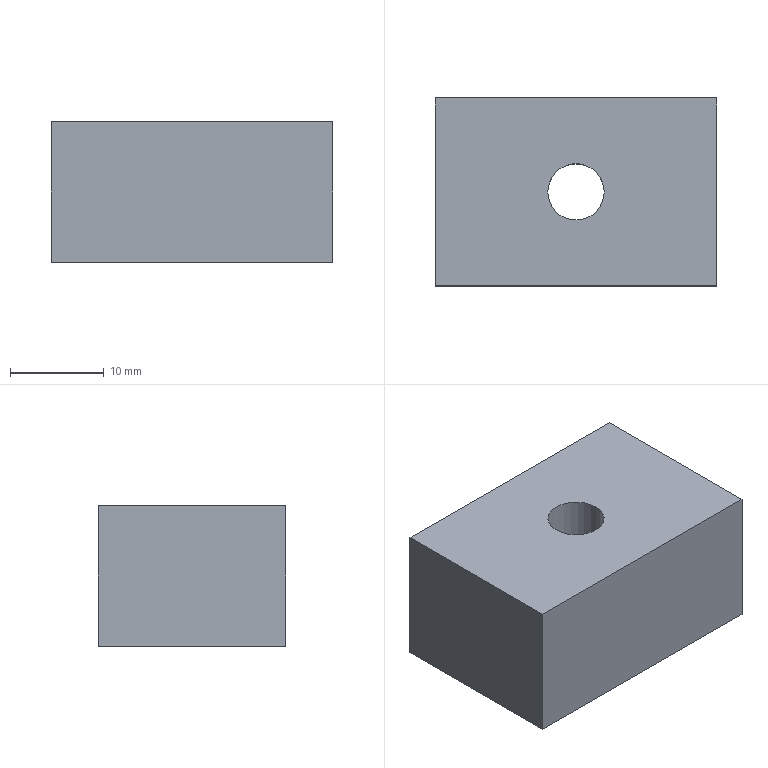Part | SolidWorks | features Extrusion 1, ICE 1 | 1 solid | 8 faces | box 30 x 20 x 15 mm | volume 8576 mm3 | plane 6 | cylinder 2 | commonest cylinder face diameters 6 x2
STEP:
#1=CARTESIAN_POINT('',(-3.,0.,0.));
#2=VERTEX_POINT('',#1);
#3=CARTESIAN_POINT('',(3.,0.,0.));
#4=VERTEX_POINT('',#3);
#5=CARTESIAN_POINT('',(0.,0.,0.));
#6=DIRECTION('',(0.,0.,1.));
#7=DIRECTION('',(1.,0.,0.));
#8=AXIS2_PLACEMENT_3D('',#5,#6,#7);
#9=CIRCLE('',#8,3.);
#10=EDGE_CURVE('',#2,#4,#9,.T.);
#11=ORIENTED_EDGE('',*,*,#10,.F.);
#12=CARTESIAN_POINT('',(-3.,0.,15.));
#13=VERTEX_POINT('',#12);
#14=CARTESIAN_POINT('',(-3.,0.,0.));
#15=DIRECTION('',(0.,0.,1.));
#16=VECTOR('',#15,1000.);
#17=LINE('',#14,#16);
#18=EDGE_CURVE('',#2,#13,#17,.T.);
#19=ORIENTED_EDGE('',*,*,#18,.T.);
#20=CARTESIAN_POINT('',(3.,0.,15.));
#21=VERTEX_POINT('',#20);
#22=CARTESIAN_POINT('',(0.,0.,15.));
#23=DIRECTION('',(0.,0.,1.));
#24=DIRECTION('',(1.,0.,0.));
#25=AXIS2_PLACEMENT_3D('',#22,#23,#24);
#26=CIRCLE('',#25,3.);
#27=EDGE_CURVE('',#13,#21,#26,.T.);
#28=ORIENTED_EDGE('',*,*,#27,.T.);
#29=CARTESIAN_POINT('',(3.,0.,0.));
#30=DIRECTION('',(0.,0.,1.));
#31=VECTOR('',#30,1000.);
#32=LINE('',#29,#31);
#33=EDGE_CURVE('',#4,#21,#32,.T.);
#34=ORIENTED_EDGE('',*,*,#33,.F.);
#35=EDGE_LOOP('',(#11,#19,#28,#34));
#36=FACE_OUTER_BOUND('',#35,.T.);
#37=CARTESIAN_POINT('',(0.,0.,0.));
#38=DIRECTION('',(0.,0.,1.));
#39=DIRECTION('',(1.,0.,0.));
#40=AXIS2_PLACEMENT_3D('',#37,#38,#39);
#41=CYLINDRICAL_SURFACE('',#40,3.);
#42=ADVANCED_FACE('',(#36),#41,.F.);
#43=CARTESIAN_POINT('',(15.,-10.,0.));
#44=VERTEX_POINT('',#43);
#45=CARTESIAN_POINT('',(15.,10.,0.));
#46=VERTEX_POINT('',#45);
#47=CARTESIAN_POINT('',(15.,10.,0.));
#48=DIRECTION('',(0.,1.,0.));
#49=VECTOR('',#48,1000.);
#50=LINE('',#47,#49);
#51=EDGE_CURVE('',#44,#46,#50,.T.);
#52=ORIENTED_EDGE('',*,*,#51,.T.);
#53=CARTESIAN_POINT('',(15.,10.,15.));
#54=VERTEX_POINT('',#53);
#55=CARTESIAN_POINT('',(15.,10.,15.));
#56=DIRECTION('',(0.,0.,-1.));
#57=VECTOR('',#56,1000.);
#58=LINE('',#55,#57);
#59=EDGE_CURVE('',#54,#46,#58,.T.);
#60=ORIENTED_EDGE('',*,*,#59,.F.);
#61=CARTESIAN_POINT('',(15.,-10.,15.));
#62=VERTEX_POINT('',#61);
#63=CARTESIAN_POINT('',(15.,10.,15.));
#64=DIRECTION('',(0.,1.,0.));
#65=VECTOR('',#64,1000.);
#66=LINE('',#63,#65);
#67=EDGE_CURVE('',#62,#54,#66,.T.);
#68=ORIENTED_EDGE('',*,*,#67,.F.);
#69=CARTESIAN_POINT('',(15.,-10.,15.));
#70=DIRECTION('',(0.,0.,-1.));
#71=VECTOR('',#70,1000.);
#72=LINE('',#69,#71);
#73=EDGE_CURVE('',#62,#44,#72,.T.);
#74=ORIENTED_EDGE('',*,*,#73,.T.);
#75=EDGE_LOOP('',(#52,#60,#68,#74));
#76=FACE_OUTER_BOUND('',#75,.T.);
#77=CARTESIAN_POINT('',(15.,10.,15.));
#78=DIRECTION('',(-1.,0.,0.));
#79=DIRECTION('',(0.,-1.,0.));
#80=AXIS2_PLACEMENT_3D('',#77,#78,#79);
#81=PLANE('',#80);
#82=ADVANCED_FACE('',(#76),#81,.F.);
#83=CARTESIAN_POINT('',(-15.,10.,0.));
#84=VERTEX_POINT('',#83);
#85=CARTESIAN_POINT('',(-15.,10.,0.));
#86=DIRECTION('',(-1.,0.,0.));
#87=VECTOR('',#86,1000.);
#88=LINE('',#85,#87);
#89=EDGE_CURVE('',#46,#84,#88,.T.);
#90=ORIENTED_EDGE('',*,*,#89,.T.);
#91=CARTESIAN_POINT('',(-15.,10.,15.));
#92=VERTEX_POINT('',#91);
#93=CARTESIAN_POINT('',(-15.,10.,15.));
#94=DIRECTION('',(0.,0.,-1.));
#95=VECTOR('',#94,1000.);
#96=LINE('',#93,#95);
#97=EDGE_CURVE('',#92,#84,#96,.T.);
#98=ORIENTED_EDGE('',*,*,#97,.F.);
#99=CARTESIAN_POINT('',(-15.,10.,15.));
#100=DIRECTION('',(-1.,0.,0.));
#101=VECTOR('',#100,1000.);
#102=LINE('',#99,#101);
#103=EDGE_CURVE('',#54,#92,#102,.T.);
#104=ORIENTED_EDGE('',*,*,#103,.F.);
#105=ORIENTED_EDGE('',*,*,#59,.T.);
#106=EDGE_LOOP('',(#90,#98,#104,#105));
#107=FACE_OUTER_BOUND('',#106,.T.);
#108=CARTESIAN_POINT('',(-15.,10.,15.));
#109=DIRECTION('',(0.,-1.,0.));
#110=DIRECTION('',(0.,0.,-1.));
#111=AXIS2_PLACEMENT_3D('',#108,#109,#110);
#112=PLANE('',#111);
#113=ADVANCED_FACE('',(#107),#112,.F.);
#114=CARTESIAN_POINT('',(-15.,-10.,0.));
#115=VERTEX_POINT('',#114);
#116=CARTESIAN_POINT('',(-15.,10.,0.));
#117=DIRECTION('',(0.,-1.,0.));
#118=VECTOR('',#117,1000.);
#119=LINE('',#116,#118);
#120=EDGE_CURVE('',#84,#115,#119,.T.);
#121=ORIENTED_EDGE('',*,*,#120,.T.);
#122=CARTESIAN_POINT('',(-15.,-10.,15.));
#123=VERTEX_POINT('',#122);
#124=CARTESIAN_POINT('',(-15.,-10.,15.));
#125=DIRECTION('',(0.,0.,-1.));
#126=VECTOR('',#125,1000.);
#127=LINE('',#124,#126);
#128=EDGE_CURVE('',#123,#115,#127,.T.);
#129=ORIENTED_EDGE('',*,*,#128,.F.);
#130=CARTESIAN_POINT('',(-15.,10.,15.));
#131=DIRECTION('',(0.,-1.,0.));
#132=VECTOR('',#131,1000.);
#133=LINE('',#130,#132);
#134=EDGE_CURVE('',#92,#123,#133,.T.);
#135=ORIENTED_EDGE('',*,*,#134,.F.);
#136=ORIENTED_EDGE('',*,*,#97,.T.);
#137=EDGE_LOOP('',(#121,#129,#135,#136));
#138=FACE_OUTER_BOUND('',#137,.T.);
#139=CARTESIAN_POINT('',(-15.,10.,15.));
#140=DIRECTION('',(1.,0.,0.));
#141=DIRECTION('',(0.,1.,0.));
#142=AXIS2_PLACEMENT_3D('',#139,#140,#141);
#143=PLANE('',#142);
#144=ADVANCED_FACE('',(#138),#143,.F.);
#145=CARTESIAN_POINT('',(-15.,-10.,0.));
#146=DIRECTION('',(1.,0.,0.));
#147=VECTOR('',#146,1000.);
#148=LINE('',#145,#147);
#149=EDGE_CURVE('',#115,#44,#148,.T.);
#150=ORIENTED_EDGE('',*,*,#149,.T.);
#151=ORIENTED_EDGE('',*,*,#73,.F.);
#152=CARTESIAN_POINT('',(-15.,-10.,15.));
#153=DIRECTION('',(1.,0.,0.));
#154=VECTOR('',#153,1000.);
#155=LINE('',#152,#154);
#156=EDGE_CURVE('',#123,#62,#155,.T.);
#157=ORIENTED_EDGE('',*,*,#156,.F.);
#158=ORIENTED_EDGE('',*,*,#128,.T.);
#159=EDGE_LOOP('',(#150,#151,#157,#158));
#160=FACE_OUTER_BOUND('',#159,.T.);
#161=CARTESIAN_POINT('',(-15.,-10.,15.));
#162=DIRECTION('',(0.,1.,0.));
#163=DIRECTION('',(0.,0.,1.));
#164=AXIS2_PLACEMENT_3D('',#161,#162,#163);
#165=PLANE('',#164);
#166=ADVANCED_FACE('',(#160),#165,.F.);
#167=CARTESIAN_POINT('',(0.,0.,15.));
#168=DIRECTION('',(0.,0.,1.));
#169=DIRECTION('',(1.,0.,0.));
#170=AXIS2_PLACEMENT_3D('',#167,#168,#169);
#171=CIRCLE('',#170,3.);
#172=EDGE_CURVE('',#21,#13,#171,.T.);
#173=ORIENTED_EDGE('',*,*,#172,.F.);
#174=ORIENTED_EDGE('',*,*,#27,.F.);
#175=EDGE_LOOP('',(#173,#174));
#176=FACE_BOUND('',#175,.T.);
#177=ORIENTED_EDGE('',*,*,#67,.T.);
#178=ORIENTED_EDGE('',*,*,#103,.T.);
#179=ORIENTED_EDGE('',*,*,#134,.T.);
#180=ORIENTED_EDGE('',*,*,#156,.T.);
#181=EDGE_LOOP('',(#177,#178,#179,#180));
#182=FACE_OUTER_BOUND('',#181,.T.);
#183=CARTESIAN_POINT('',(0.,0.,15.));
#184=DIRECTION('',(0.,0.,1.));
#185=DIRECTION('',(1.,0.,0.));
#186=AXIS2_PLACEMENT_3D('',#183,#184,#185);
#187=PLANE('',#186);
#188=ADVANCED_FACE('',(#176,#182),#187,.T.);
#189=CARTESIAN_POINT('',(0.,0.,0.));
#190=DIRECTION('',(0.,0.,1.));
#191=DIRECTION('',(1.,0.,0.));
#192=AXIS2_PLACEMENT_3D('',#189,#190,#191);
#193=CIRCLE('',#192,3.);
#194=EDGE_CURVE('',#4,#2,#193,.T.);
#195=ORIENTED_EDGE('',*,*,#194,.T.);
#196=ORIENTED_EDGE('',*,*,#10,.T.);
#197=EDGE_LOOP('',(#195,#196));
#198=FACE_BOUND('',#197,.T.);
#199=ORIENTED_EDGE('',*,*,#51,.F.);
#200=ORIENTED_EDGE('',*,*,#149,.F.);
#201=ORIENTED_EDGE('',*,*,#120,.F.);
#202=ORIENTED_EDGE('',*,*,#89,.F.);
#203=EDGE_LOOP('',(#199,#200,#201,#202));
#204=FACE_OUTER_BOUND('',#203,.T.);
#205=CARTESIAN_POINT('',(0.,0.,0.));
#206=DIRECTION('',(0.,0.,1.));
#207=DIRECTION('',(1.,0.,0.));
#208=AXIS2_PLACEMENT_3D('',#205,#206,#207);
#209=PLANE('',#208);
#210=ADVANCED_FACE('',(#198,#204),#209,.F.);
#211=ORIENTED_EDGE('',*,*,#18,.F.);
#212=ORIENTED_EDGE('',*,*,#194,.F.);
#213=ORIENTED_EDGE('',*,*,#33,.T.);
#214=ORIENTED_EDGE('',*,*,#172,.T.);
#215=EDGE_LOOP('',(#211,#212,#213,#214));
#216=FACE_OUTER_BOUND('',#215,.T.);
#217=CARTESIAN_POINT('',(0.,0.,0.));
#218=DIRECTION('',(0.,0.,1.));
#219=DIRECTION('',(1.,0.,0.));
#220=AXIS2_PLACEMENT_3D('',#217,#218,#219);
#221=CYLINDRICAL_SURFACE('',#220,3.);
#222=ADVANCED_FACE('',(#216),#221,.F.);
#223=CLOSED_SHELL('',(#42,#82,#113,#144,#166,#188,#210,#222));
#224=MANIFOLD_SOLID_BREP('',#223);
#225=CARTESIAN_POINT('',(0.,0.,0.));
#226=DIRECTION('',(0.,0.,1.));
#227=DIRECTION('',(1.,0.,0.));
#228=AXIS2_PLACEMENT_3D('',#225,#226,#227);
#229=(LENGTH_UNIT()NAMED_UNIT(*)SI_UNIT(.MILLI.,.METRE.));
#230=UNCERTAINTY_MEASURE_WITH_UNIT(LENGTH_MEASURE(0.00001),#229,'','');
#231=(NAMED_UNIT(*)PLANE_ANGLE_UNIT()SI_UNIT($,.RADIAN.));
#232=(NAMED_UNIT(*)SI_UNIT($,.STERADIAN.)SOLID_ANGLE_UNIT());
#233=(GEOMETRIC_REPRESENTATION_CONTEXT(3)GLOBAL_UNCERTAINTY_ASSIGNED_CONTEXT((#230))GLOBAL_UNIT_ASSIGNED_CONTEXT((#229,#231,#232))REPRESENTATION_CONTEXT('',''));
#234=ADVANCED_BREP_SHAPE_REPRESENTATION('',(#224,#228),#233);